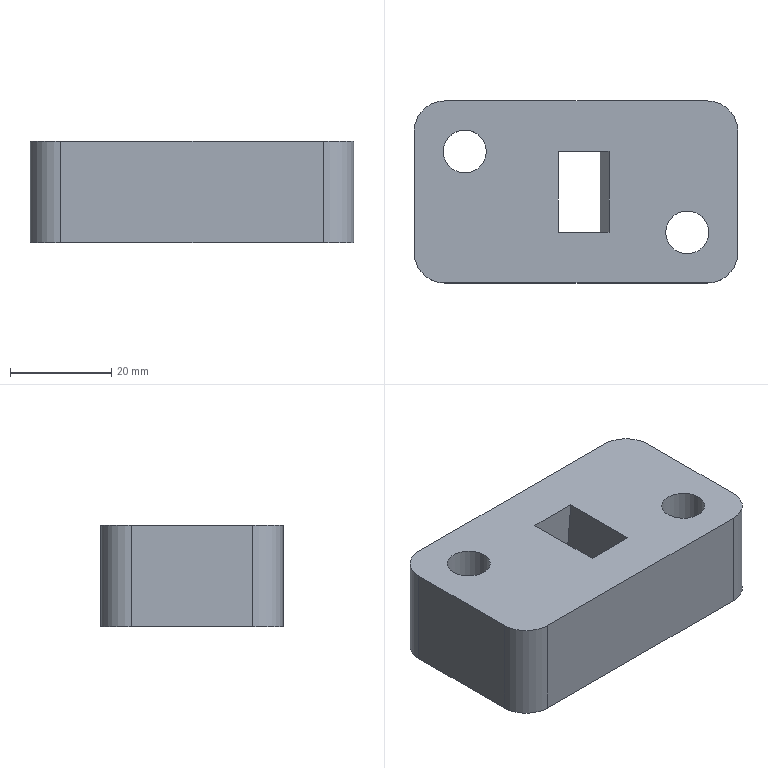Part | STEP file | solid 97 | 1 solid | 38 faces | box 64 x 36 x 20 mm | volume 38229 mm3 | plane 26 | cylinder 8 | other 4 | commonest cylinder face diameters 12 x4 8.5 x2 14 x2